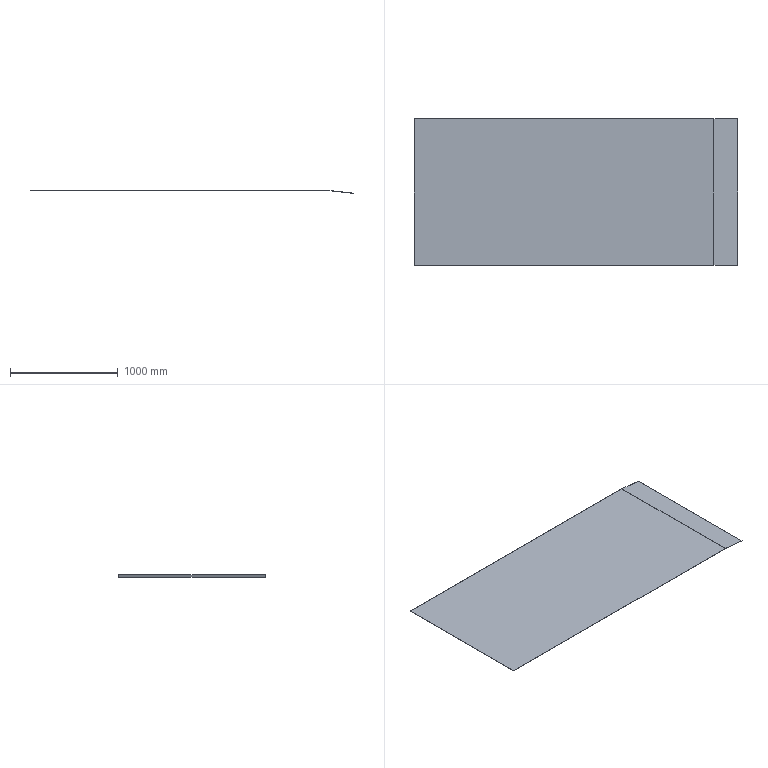Part | STEP file | VD-SYL0380DJ1006_1_1-6_VD-SYL03 | 1 solid | 10 faces | box 2999 x 1359 x 24.985 mm | volume 8157094 mm3 | plane 10
STEP:
#1=CARTESIAN_POINT('',(-1441.712,-679.5,0.));
#2=VERTEX_POINT('',#1);
#3=CARTESIAN_POINT('',(-1441.712,-679.5,2.));
#4=VERTEX_POINT('',#3);
#5=CARTESIAN_POINT('',(-1441.712,-679.5,0.));
#6=DIRECTION('',(0.,0.,1.));
#7=VECTOR('',#6,1000.);
#8=LINE('',#5,#7);
#9=EDGE_CURVE('',#2,#4,#8,.T.);
#10=ORIENTED_EDGE('',*,*,#9,.T.);
#11=CARTESIAN_POINT('',(-1441.712,679.5,2.));
#12=VERTEX_POINT('',#11);
#13=CARTESIAN_POINT('',(-1441.712,679.5,2.));
#14=DIRECTION('',(0.,-1.,0.));
#15=VECTOR('',#14,1000.);
#16=LINE('',#13,#15);
#17=EDGE_CURVE('',#12,#4,#16,.T.);
#18=ORIENTED_EDGE('',*,*,#17,.F.);
#19=CARTESIAN_POINT('',(-1441.712,679.5,0.));
#20=VERTEX_POINT('',#19);
#21=CARTESIAN_POINT('',(-1441.712,679.5,0.));
#22=DIRECTION('',(0.,0.,1.));
#23=VECTOR('',#22,1000.);
#24=LINE('',#21,#23);
#25=EDGE_CURVE('',#20,#12,#24,.T.);
#26=ORIENTED_EDGE('',*,*,#25,.F.);
#27=CARTESIAN_POINT('',(-1441.712,679.5,0.));
#28=DIRECTION('',(0.,-1.,0.));
#29=VECTOR('',#28,1000.);
#30=LINE('',#27,#29);
#31=EDGE_CURVE('',#20,#2,#30,.T.);
#32=ORIENTED_EDGE('',*,*,#31,.T.);
#33=EDGE_LOOP('',(#10,#18,#26,#32));
#34=FACE_OUTER_BOUND('',#33,.T.);
#35=CARTESIAN_POINT('',(-1441.712,0.,1.));
#36=DIRECTION('',(1.,0.,0.));
#37=DIRECTION('',(0.,1.,0.));
#38=AXIS2_PLACEMENT_3D('',#35,#36,#37);
#39=PLANE('',#38);
#40=ADVANCED_FACE('',(#34),#39,.F.);
#41=ORIENTED_EDGE('',*,*,#25,.T.);
#42=CARTESIAN_POINT('',(1338.913,679.5,2.));
#43=VERTEX_POINT('',#42);
#44=CARTESIAN_POINT('',(-1441.712,679.5,2.));
#45=DIRECTION('',(1.,0.,0.));
#46=VECTOR('',#45,1000.);
#47=LINE('',#44,#46);
#48=EDGE_CURVE('',#12,#43,#47,.T.);
#49=ORIENTED_EDGE('',*,*,#48,.T.);
#50=CARTESIAN_POINT('',(1338.86,679.5,0.000015));
#51=VERTEX_POINT('',#50);
#52=CARTESIAN_POINT('',(1338.86,679.5,0.000015));
#53=DIRECTION('',(0.02627,0.,0.9997));
#54=VECTOR('',#53,1000.);
#55=LINE('',#52,#54);
#56=EDGE_CURVE('',#51,#43,#55,.T.);
#57=ORIENTED_EDGE('',*,*,#56,.F.);
#58=CARTESIAN_POINT('',(-1441.712,679.5,0.));
#59=CARTESIAN_POINT('',(-514.855,679.5,0.));
#60=CARTESIAN_POINT('',(412.003,679.5,0.));
#61=CARTESIAN_POINT('',(1338.86,679.5,0.000015));
#62=B_SPLINE_CURVE_WITH_KNOTS('',3,(#58,#59,#60,#61),.UNSPECIFIED.,.F.,.F.,(4,4),(0.,1.),.UNSPECIFIED.);
#63=EDGE_CURVE('',#20,#51,#62,.T.);
#64=ORIENTED_EDGE('',*,*,#63,.F.);
#65=EDGE_LOOP('',(#41,#49,#57,#64));
#66=FACE_OUTER_BOUND('',#65,.T.);
#67=CARTESIAN_POINT('',(-51.4,679.5,1.));
#68=DIRECTION('',(0.,1.,0.));
#69=DIRECTION('',(1.,0.,0.));
#70=AXIS2_PLACEMENT_3D('',#67,#68,#69);
#71=PLANE('',#70);
#72=ADVANCED_FACE('',(#66),#71,.T.);
#73=CARTESIAN_POINT('',(1338.86,-679.5,0.000015));
#74=VERTEX_POINT('',#73);
#75=CARTESIAN_POINT('',(1338.913,-679.5,2.));
#76=VERTEX_POINT('',#75);
#77=CARTESIAN_POINT('',(1338.86,-679.5,0.000015));
#78=DIRECTION('',(0.02627,0.,0.9997));
#79=VECTOR('',#78,1000.);
#80=LINE('',#77,#79);
#81=EDGE_CURVE('',#74,#76,#80,.T.);
#82=ORIENTED_EDGE('',*,*,#81,.F.);
#83=CARTESIAN_POINT('',(1557.498,-679.5,-22.985));
#84=VERTEX_POINT('',#83);
#85=CARTESIAN_POINT('',(1338.86,-679.5,0.000015));
#86=CARTESIAN_POINT('',(1411.739,-679.5,-7.662));
#87=CARTESIAN_POINT('',(1484.619,-679.5,-15.324));
#88=CARTESIAN_POINT('',(1557.498,-679.5,-22.985));
#89=B_SPLINE_CURVE_WITH_KNOTS('',3,(#85,#86,#87,#88),.UNSPECIFIED.,.F.,.F.,(4,4),(0.,1.),.UNSPECIFIED.);
#90=EDGE_CURVE('',#74,#84,#89,.T.);
#91=ORIENTED_EDGE('',*,*,#90,.T.);
#92=CARTESIAN_POINT('',(1557.707,-679.5,-20.996));
#93=VERTEX_POINT('',#92);
#94=CARTESIAN_POINT('',(1557.707,-679.5,-20.996));
#95=DIRECTION('',(-0.1045,0.,-0.9945));
#96=VECTOR('',#95,1000.);
#97=LINE('',#94,#96);
#98=EDGE_CURVE('',#93,#84,#97,.T.);
#99=ORIENTED_EDGE('',*,*,#98,.F.);
#100=CARTESIAN_POINT('',(1338.913,-679.5,2.));
#101=DIRECTION('',(0.9945,0.,-0.1045));
#102=VECTOR('',#101,1000.);
#103=LINE('',#100,#102);
#104=EDGE_CURVE('',#76,#93,#103,.T.);
#105=ORIENTED_EDGE('',*,*,#104,.F.);
#106=EDGE_LOOP('',(#82,#91,#99,#105));
#107=FACE_OUTER_BOUND('',#106,.T.);
#108=CARTESIAN_POINT('',(1448.257,-679.5,-10.498));
#109=DIRECTION('',(0.,-1.,0.));
#110=DIRECTION('',(0.,0.,-1.));
#111=AXIS2_PLACEMENT_3D('',#108,#109,#110);
#112=PLANE('',#111);
#113=ADVANCED_FACE('',(#107),#112,.T.);
#114=ORIENTED_EDGE('',*,*,#98,.T.);
#115=CARTESIAN_POINT('',(1557.498,679.5,-22.985));
#116=VERTEX_POINT('',#115);
#117=CARTESIAN_POINT('',(1557.498,679.5,-22.985));
#118=DIRECTION('',(0.,-1.,0.));
#119=VECTOR('',#118,1000.);
#120=LINE('',#117,#119);
#121=EDGE_CURVE('',#116,#84,#120,.T.);
#122=ORIENTED_EDGE('',*,*,#121,.F.);
#123=CARTESIAN_POINT('',(1557.707,679.5,-20.996));
#124=VERTEX_POINT('',#123);
#125=CARTESIAN_POINT('',(1557.707,679.5,-20.996));
#126=DIRECTION('',(-0.1045,0.,-0.9945));
#127=VECTOR('',#126,1000.);
#128=LINE('',#125,#127);
#129=EDGE_CURVE('',#124,#116,#128,.T.);
#130=ORIENTED_EDGE('',*,*,#129,.F.);
#131=CARTESIAN_POINT('',(1557.707,679.5,-20.996));
#132=DIRECTION('',(0.,-1.,0.));
#133=VECTOR('',#132,1000.);
#134=LINE('',#131,#133);
#135=EDGE_CURVE('',#124,#93,#134,.T.);
#136=ORIENTED_EDGE('',*,*,#135,.T.);
#137=EDGE_LOOP('',(#114,#122,#130,#136));
#138=FACE_OUTER_BOUND('',#137,.T.);
#139=CARTESIAN_POINT('',(1557.603,0.,-21.991));
#140=DIRECTION('',(-0.9945,0.,0.1045));
#141=DIRECTION('',(0.,1.,0.));
#142=AXIS2_PLACEMENT_3D('',#139,#140,#141);
#143=PLANE('',#142);
#144=ADVANCED_FACE('',(#138),#143,.F.);
#145=CARTESIAN_POINT('',(1338.913,679.5,2.));
#146=DIRECTION('',(0.,-1.,0.));
#147=VECTOR('',#146,1000.);
#148=LINE('',#145,#147);
#149=EDGE_CURVE('',#43,#76,#148,.T.);
#150=ORIENTED_EDGE('',*,*,#149,.T.);
#151=ORIENTED_EDGE('',*,*,#104,.T.);
#152=ORIENTED_EDGE('',*,*,#135,.F.);
#153=CARTESIAN_POINT('',(1338.913,679.5,2.));
#154=DIRECTION('',(0.9945,0.,-0.1045));
#155=VECTOR('',#154,1000.);
#156=LINE('',#153,#155);
#157=EDGE_CURVE('',#43,#124,#156,.T.);
#158=ORIENTED_EDGE('',*,*,#157,.F.);
#159=EDGE_LOOP('',(#150,#151,#152,#158));
#160=FACE_OUTER_BOUND('',#159,.T.);
#161=CARTESIAN_POINT('',(1338.913,679.5,2.));
#162=DIRECTION('',(-0.1045,0.,-0.9945));
#163=DIRECTION('',(-0.9945,0.,0.1045));
#164=AXIS2_PLACEMENT_3D('',#161,#162,#163);
#165=PLANE('',#164);
#166=ADVANCED_FACE('',(#160),#165,.F.);
#167=ORIENTED_EDGE('',*,*,#129,.T.);
#168=CARTESIAN_POINT('',(1338.86,679.5,0.000015));
#169=CARTESIAN_POINT('',(1411.739,679.5,-7.665));
#170=CARTESIAN_POINT('',(1484.619,679.5,-15.325));
#171=CARTESIAN_POINT('',(1557.498,679.5,-22.985));
#172=B_SPLINE_CURVE_WITH_KNOTS('',3,(#168,#169,#170,#171),.UNSPECIFIED.,.F.,.F.,(4,4),(0.,1.),.UNSPECIFIED.);
#173=EDGE_CURVE('',#51,#116,#172,.T.);
#174=ORIENTED_EDGE('',*,*,#173,.F.);
#175=ORIENTED_EDGE('',*,*,#56,.T.);
#176=ORIENTED_EDGE('',*,*,#157,.T.);
#177=EDGE_LOOP('',(#167,#174,#175,#176));
#178=FACE_OUTER_BOUND('',#177,.T.);
#179=CARTESIAN_POINT('',(1448.257,679.5,-10.498));
#180=DIRECTION('',(0.,-1.,0.));
#181=DIRECTION('',(0.,0.,-1.));
#182=AXIS2_PLACEMENT_3D('',#179,#180,#181);
#183=PLANE('',#182);
#184=ADVANCED_FACE('',(#178),#183,.F.);
#185=ORIENTED_EDGE('',*,*,#121,.T.);
#186=ORIENTED_EDGE('',*,*,#90,.F.);
#187=CARTESIAN_POINT('',(1338.86,679.5,0.000015));
#188=CARTESIAN_POINT('',(1338.86,226.5,0.));
#189=CARTESIAN_POINT('',(1338.86,-226.5,0.));
#190=CARTESIAN_POINT('',(1338.86,-679.5,0.000015));
#191=B_SPLINE_CURVE_WITH_KNOTS('',3,(#187,#188,#189,#190),.UNSPECIFIED.,.F.,.F.,(4,4),(0.,1.),.UNSPECIFIED.);
#192=EDGE_CURVE('',#51,#74,#191,.T.);
#193=ORIENTED_EDGE('',*,*,#192,.F.);
#194=ORIENTED_EDGE('',*,*,#173,.T.);
#195=EDGE_LOOP('',(#185,#186,#193,#194));
#196=FACE_OUTER_BOUND('',#195,.T.);
#197=CARTESIAN_POINT('',(1338.703,679.5,0.01096));
#198=DIRECTION('',(-0.1045,0.,-0.9945));
#199=DIRECTION('',(-0.9945,0.,0.1045));
#200=AXIS2_PLACEMENT_3D('',#197,#198,#199);
#201=PLANE('',#200);
#202=ADVANCED_FACE('',(#196),#201,.T.);
#203=CARTESIAN_POINT('',(1338.86,-679.5,0.000015));
#204=CARTESIAN_POINT('',(412.003,-679.5,0.));
#205=CARTESIAN_POINT('',(-514.855,-679.5,0.));
#206=CARTESIAN_POINT('',(-1441.712,-679.5,0.));
#207=B_SPLINE_CURVE_WITH_KNOTS('',3,(#203,#204,#205,#206),.UNSPECIFIED.,.F.,.F.,(4,4),(0.,1.),.UNSPECIFIED.);
#208=EDGE_CURVE('',#74,#2,#207,.T.);
#209=ORIENTED_EDGE('',*,*,#208,.T.);
#210=ORIENTED_EDGE('',*,*,#31,.F.);
#211=ORIENTED_EDGE('',*,*,#63,.T.);
#212=ORIENTED_EDGE('',*,*,#192,.T.);
#213=EDGE_LOOP('',(#209,#210,#211,#212));
#214=FACE_OUTER_BOUND('',#213,.T.);
#215=CARTESIAN_POINT('',(0.,0.,0.));
#216=DIRECTION('',(0.,0.,1.));
#217=DIRECTION('',(1.,0.,0.));
#218=AXIS2_PLACEMENT_3D('',#215,#216,#217);
#219=PLANE('',#218);
#220=ADVANCED_FACE('',(#214),#219,.F.);
#221=ORIENTED_EDGE('',*,*,#81,.T.);
#222=CARTESIAN_POINT('',(1338.913,-679.5,2.));
#223=DIRECTION('',(-1.,0.,0.));
#224=VECTOR('',#223,1000.);
#225=LINE('',#222,#224);
#226=EDGE_CURVE('',#76,#4,#225,.T.);
#227=ORIENTED_EDGE('',*,*,#226,.T.);
#228=ORIENTED_EDGE('',*,*,#9,.F.);
#229=ORIENTED_EDGE('',*,*,#208,.F.);
#230=EDGE_LOOP('',(#221,#227,#228,#229));
#231=FACE_OUTER_BOUND('',#230,.T.);
#232=CARTESIAN_POINT('',(-51.4,-679.5,1.));
#233=DIRECTION('',(0.,-1.,0.));
#234=DIRECTION('',(0.,0.,-1.));
#235=AXIS2_PLACEMENT_3D('',#232,#233,#234);
#236=PLANE('',#235);
#237=ADVANCED_FACE('',(#231),#236,.T.);
#238=ORIENTED_EDGE('',*,*,#149,.F.);
#239=ORIENTED_EDGE('',*,*,#48,.F.);
#240=ORIENTED_EDGE('',*,*,#17,.T.);
#241=ORIENTED_EDGE('',*,*,#226,.F.);
#242=EDGE_LOOP('',(#238,#239,#240,#241));
#243=FACE_OUTER_BOUND('',#242,.T.);
#244=CARTESIAN_POINT('',(0.,0.,2.));
#245=DIRECTION('',(0.,0.,1.));
#246=DIRECTION('',(1.,0.,0.));
#247=AXIS2_PLACEMENT_3D('',#244,#245,#246);
#248=PLANE('',#247);
#249=ADVANCED_FACE('',(#243),#248,.T.);
#250=CLOSED_SHELL('',(#40,#72,#113,#144,#166,#184,#202,#220,#237,#249));
#251=MANIFOLD_SOLID_BREP('',#250);
#252=CARTESIAN_POINT('',(0.,0.,0.));
#253=DIRECTION('',(0.,0.,1.));
#254=DIRECTION('',(1.,0.,0.));
#255=AXIS2_PLACEMENT_3D('',#252,#253,#254);
#256=(LENGTH_UNIT()NAMED_UNIT(*)SI_UNIT(.MILLI.,.METRE.));
#257=UNCERTAINTY_MEASURE_WITH_UNIT(LENGTH_MEASURE(0.00001),#256,'','');
#258=(NAMED_UNIT(*)PLANE_ANGLE_UNIT()SI_UNIT($,.RADIAN.));
#259=(NAMED_UNIT(*)SI_UNIT($,.STERADIAN.)SOLID_ANGLE_UNIT());
#260=(GEOMETRIC_REPRESENTATION_CONTEXT(3)GLOBAL_UNCERTAINTY_ASSIGNED_CONTEXT((#257))GLOBAL_UNIT_ASSIGNED_CONTEXT((#256,#258,#259))REPRESENTATION_CONTEXT('',''));
#261=ADVANCED_BREP_SHAPE_REPRESENTATION('',(#251,#255),#260);